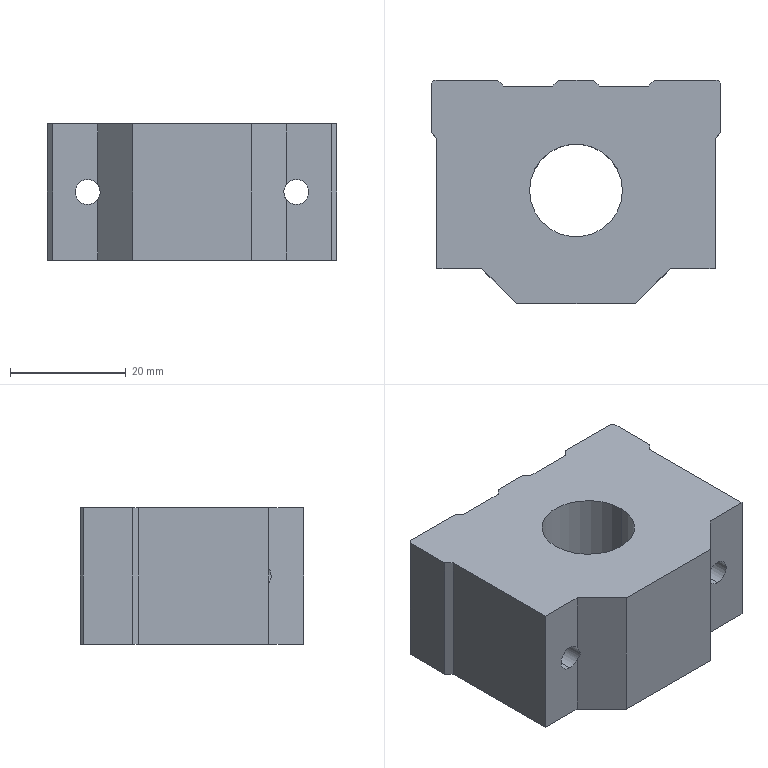Part | SolidWorks | features Extrusion 1, ICE 1 | 1 solid | 30 faces | box 50 x 38.5 x 23.5 mm | volume 34722 mm3 | plane 24 | cylinder 6 | commonest cylinder face diameters 4.3 x4 16 x2
STEP:
#1=CARTESIAN_POINT('',(18.,-13.5,9.6));
#2=VERTEX_POINT('',#1);
#3=CARTESIAN_POINT('',(16.25,-13.5,10.501));
#4=VERTEX_POINT('',#3);
#5=CARTESIAN_POINT('',(18.,-13.5,11.75));
#6=DIRECTION('',(0.,1.,0.));
#7=DIRECTION('',(0.,0.,1.));
#8=AXIS2_PLACEMENT_3D('',#5,#6,#7);
#9=CIRCLE('',#8,2.15);
#10=EDGE_CURVE('',#2,#4,#9,.T.);
#11=ORIENTED_EDGE('',*,*,#10,.F.);
#12=CARTESIAN_POINT('',(18.,19.,9.6));
#13=VERTEX_POINT('',#12);
#14=CARTESIAN_POINT('',(18.,-19.5,9.6));
#15=DIRECTION('',(0.,1.,0.));
#16=VECTOR('',#15,1000.);
#17=LINE('',#14,#16);
#18=EDGE_CURVE('',#2,#13,#17,.T.);
#19=ORIENTED_EDGE('',*,*,#18,.T.);
#20=CARTESIAN_POINT('',(18.,19.,13.9));
#21=VERTEX_POINT('',#20);
#22=CARTESIAN_POINT('',(18.,19.,11.75));
#23=DIRECTION('',(0.,1.,0.));
#24=DIRECTION('',(0.,0.,1.));
#25=AXIS2_PLACEMENT_3D('',#22,#23,#24);
#26=CIRCLE('',#25,2.15);
#27=EDGE_CURVE('',#13,#21,#26,.T.);
#28=ORIENTED_EDGE('',*,*,#27,.T.);
#29=CARTESIAN_POINT('',(18.,-13.5,13.9));
#30=VERTEX_POINT('',#29);
#31=CARTESIAN_POINT('',(18.,-19.5,13.9));
#32=DIRECTION('',(0.,1.,0.));
#33=VECTOR('',#32,1000.);
#34=LINE('',#31,#33);
#35=EDGE_CURVE('',#30,#21,#34,.T.);
#36=ORIENTED_EDGE('',*,*,#35,.F.);
#37=CARTESIAN_POINT('',(16.25,-13.5,12.999));
#38=VERTEX_POINT('',#37);
#39=CARTESIAN_POINT('',(18.,-13.5,11.75));
#40=DIRECTION('',(0.,1.,0.));
#41=DIRECTION('',(0.,0.,1.));
#42=AXIS2_PLACEMENT_3D('',#39,#40,#41);
#43=CIRCLE('',#42,2.15);
#44=EDGE_CURVE('',#38,#30,#43,.T.);
#45=ORIENTED_EDGE('',*,*,#44,.F.);
#46=CARTESIAN_POINT('',(16.25,-13.5,10.501));
#47=CARTESIAN_POINT('',(15.698,-14.052,11.275));
#48=CARTESIAN_POINT('',(15.698,-14.052,12.225));
#49=CARTESIAN_POINT('',(16.25,-13.5,12.999));
#50=(BOUNDED_CURVE()B_SPLINE_CURVE(3,(#46,#47,#48,#49),.UNSPECIFIED.,.F.,.F.)B_SPLINE_CURVE_WITH_KNOTS((4,4),(2.522,3.761),.UNSPECIFIED.)CURVE()GEOMETRIC_REPRESENTATION_ITEM()RATIONAL_B_SPLINE_CURVE((1.,0.876,0.876,1.))REPRESENTATION_ITEM(''));
#51=EDGE_CURVE('',#4,#38,#50,.T.);
#52=ORIENTED_EDGE('',*,*,#51,.F.);
#53=EDGE_LOOP('',(#11,#19,#28,#36,#45,#52));
#54=FACE_OUTER_BOUND('',#53,.T.);
#55=CARTESIAN_POINT('',(18.,-19.5,11.75));
#56=DIRECTION('',(0.,1.,0.));
#57=DIRECTION('',(0.,0.,1.));
#58=AXIS2_PLACEMENT_3D('',#55,#56,#57);
#59=CYLINDRICAL_SURFACE('',#58,2.15);
#60=ADVANCED_FACE('',(#54),#59,.F.);
#61=CARTESIAN_POINT('',(-18.,-13.5,9.6));
#62=VERTEX_POINT('',#61);
#63=CARTESIAN_POINT('',(-18.,-13.5,13.9));
#64=VERTEX_POINT('',#63);
#65=CARTESIAN_POINT('',(-18.,-13.5,11.75));
#66=DIRECTION('',(0.,1.,0.));
#67=DIRECTION('',(0.,0.,1.));
#68=AXIS2_PLACEMENT_3D('',#65,#66,#67);
#69=CIRCLE('',#68,2.15);
#70=EDGE_CURVE('',#62,#64,#69,.T.);
#71=ORIENTED_EDGE('',*,*,#70,.F.);
#72=CARTESIAN_POINT('',(-18.,19.,9.6));
#73=VERTEX_POINT('',#72);
#74=CARTESIAN_POINT('',(-18.,-19.5,9.6));
#75=DIRECTION('',(0.,1.,0.));
#76=VECTOR('',#75,1000.);
#77=LINE('',#74,#76);
#78=EDGE_CURVE('',#62,#73,#77,.T.);
#79=ORIENTED_EDGE('',*,*,#78,.T.);
#80=CARTESIAN_POINT('',(-18.,19.,13.9));
#81=VERTEX_POINT('',#80);
#82=CARTESIAN_POINT('',(-18.,19.,11.75));
#83=DIRECTION('',(0.,1.,0.));
#84=DIRECTION('',(0.,0.,1.));
#85=AXIS2_PLACEMENT_3D('',#82,#83,#84);
#86=CIRCLE('',#85,2.15);
#87=EDGE_CURVE('',#73,#81,#86,.T.);
#88=ORIENTED_EDGE('',*,*,#87,.T.);
#89=CARTESIAN_POINT('',(-18.,-19.5,13.9));
#90=DIRECTION('',(0.,1.,0.));
#91=VECTOR('',#90,1000.);
#92=LINE('',#89,#91);
#93=EDGE_CURVE('',#64,#81,#92,.T.);
#94=ORIENTED_EDGE('',*,*,#93,.F.);
#95=EDGE_LOOP('',(#71,#79,#88,#94));
#96=FACE_OUTER_BOUND('',#95,.T.);
#97=CARTESIAN_POINT('',(-18.,-19.5,11.75));
#98=DIRECTION('',(0.,1.,0.));
#99=DIRECTION('',(0.,0.,1.));
#100=AXIS2_PLACEMENT_3D('',#97,#98,#99);
#101=CYLINDRICAL_SURFACE('',#100,2.15);
#102=ADVANCED_FACE('',(#96),#101,.F.);
#103=CARTESIAN_POINT('',(-8.,0.,23.5));
#104=VERTEX_POINT('',#103);
#105=CARTESIAN_POINT('',(8.,0.,23.5));
#106=VERTEX_POINT('',#105);
#107=CARTESIAN_POINT('',(0.,0.,23.5));
#108=DIRECTION('',(0.,0.,1.));
#109=DIRECTION('',(1.,0.,0.));
#110=AXIS2_PLACEMENT_3D('',#107,#108,#109);
#111=CIRCLE('',#110,8.);
#112=EDGE_CURVE('',#104,#106,#111,.T.);
#113=ORIENTED_EDGE('',*,*,#112,.T.);
#114=CARTESIAN_POINT('',(8.,0.,0.));
#115=VERTEX_POINT('',#114);
#116=CARTESIAN_POINT('',(8.,0.,23.5));
#117=DIRECTION('',(0.,0.,-1.));
#118=VECTOR('',#117,1000.);
#119=LINE('',#116,#118);
#120=EDGE_CURVE('',#106,#115,#119,.T.);
#121=ORIENTED_EDGE('',*,*,#120,.T.);
#122=CARTESIAN_POINT('',(-8.,0.,0.));
#123=VERTEX_POINT('',#122);
#124=CARTESIAN_POINT('',(0.,0.,0.));
#125=DIRECTION('',(0.,0.,1.));
#126=DIRECTION('',(1.,0.,0.));
#127=AXIS2_PLACEMENT_3D('',#124,#125,#126);
#128=CIRCLE('',#127,8.);
#129=EDGE_CURVE('',#123,#115,#128,.T.);
#130=ORIENTED_EDGE('',*,*,#129,.F.);
#131=CARTESIAN_POINT('',(-8.,0.,23.5));
#132=DIRECTION('',(0.,0.,-1.));
#133=VECTOR('',#132,1000.);
#134=LINE('',#131,#133);
#135=EDGE_CURVE('',#104,#123,#134,.T.);
#136=ORIENTED_EDGE('',*,*,#135,.F.);
#137=EDGE_LOOP('',(#113,#121,#130,#136));
#138=FACE_OUTER_BOUND('',#137,.T.);
#139=CARTESIAN_POINT('',(0.,0.,23.5));
#140=DIRECTION('',(0.,0.,-1.));
#141=DIRECTION('',(-1.,0.,0.));
#142=AXIS2_PLACEMENT_3D('',#139,#140,#141);
#143=CYLINDRICAL_SURFACE('',#142,8.);
#144=ADVANCED_FACE('',(#138),#143,.F.);
#145=CARTESIAN_POINT('',(-16.25,-13.5,23.5));
#146=VERTEX_POINT('',#145);
#147=CARTESIAN_POINT('',(-10.25,-19.5,23.5));
#148=VERTEX_POINT('',#147);
#149=CARTESIAN_POINT('',(-16.25,-13.5,23.5));
#150=DIRECTION('',(0.7071,-0.7071,0.));
#151=VECTOR('',#150,1000.);
#152=LINE('',#149,#151);
#153=EDGE_CURVE('',#146,#148,#152,.T.);
#154=ORIENTED_EDGE('',*,*,#153,.T.);
#155=CARTESIAN_POINT('',(10.25,-19.5,23.5));
#156=VERTEX_POINT('',#155);
#157=CARTESIAN_POINT('',(-10.25,-19.5,23.5));
#158=DIRECTION('',(1.,0.,0.));
#159=VECTOR('',#158,1000.);
#160=LINE('',#157,#159);
#161=EDGE_CURVE('',#148,#156,#160,.T.);
#162=ORIENTED_EDGE('',*,*,#161,.T.);
#163=CARTESIAN_POINT('',(16.25,-13.5,23.5));
#164=VERTEX_POINT('',#163);
#165=CARTESIAN_POINT('',(16.25,-13.5,23.5));
#166=DIRECTION('',(0.7071,0.7071,0.));
#167=VECTOR('',#166,1000.);
#168=LINE('',#165,#167);
#169=EDGE_CURVE('',#156,#164,#168,.T.);
#170=ORIENTED_EDGE('',*,*,#169,.T.);
#171=CARTESIAN_POINT('',(24.,-13.5,23.5));
#172=VERTEX_POINT('',#171);
#173=CARTESIAN_POINT('',(16.25,-13.5,23.5));
#174=DIRECTION('',(1.,0.,0.));
#175=VECTOR('',#174,1000.);
#176=LINE('',#173,#175);
#177=EDGE_CURVE('',#164,#172,#176,.T.);
#178=ORIENTED_EDGE('',*,*,#177,.T.);
#179=CARTESIAN_POINT('',(24.,9.,23.5));
#180=VERTEX_POINT('',#179);
#181=CARTESIAN_POINT('',(24.,-13.5,23.5));
#182=DIRECTION('',(0.,1.,0.));
#183=VECTOR('',#182,1000.);
#184=LINE('',#181,#183);
#185=EDGE_CURVE('',#172,#180,#184,.T.);
#186=ORIENTED_EDGE('',*,*,#185,.T.);
#187=CARTESIAN_POINT('',(25.,10.,23.5));
#188=VERTEX_POINT('',#187);
#189=CARTESIAN_POINT('',(24.,9.,23.5));
#190=DIRECTION('',(0.7071,0.7071,0.));
#191=VECTOR('',#190,1000.);
#192=LINE('',#189,#191);
#193=EDGE_CURVE('',#180,#188,#192,.T.);
#194=ORIENTED_EDGE('',*,*,#193,.T.);
#195=CARTESIAN_POINT('',(25.,18.5,23.5));
#196=VERTEX_POINT('',#195);
#197=CARTESIAN_POINT('',(25.,10.,23.5));
#198=DIRECTION('',(0.,1.,0.));
#199=VECTOR('',#198,1000.);
#200=LINE('',#197,#199);
#201=EDGE_CURVE('',#188,#196,#200,.T.);
#202=ORIENTED_EDGE('',*,*,#201,.T.);
#203=CARTESIAN_POINT('',(24.5,19.,23.5));
#204=VERTEX_POINT('',#203);
#205=CARTESIAN_POINT('',(25.,18.5,23.5));
#206=DIRECTION('',(-0.7071,0.7071,0.));
#207=VECTOR('',#206,1000.);
#208=LINE('',#205,#207);
#209=EDGE_CURVE('',#196,#204,#208,.T.);
#210=ORIENTED_EDGE('',*,*,#209,.T.);
#211=CARTESIAN_POINT('',(13.5,19.,23.5));
#212=VERTEX_POINT('',#211);
#213=CARTESIAN_POINT('',(24.5,19.,23.5));
#214=DIRECTION('',(-1.,0.,0.));
#215=VECTOR('',#214,1000.);
#216=LINE('',#213,#215);
#217=EDGE_CURVE('',#204,#212,#216,.T.);
#218=ORIENTED_EDGE('',*,*,#217,.T.);
#219=CARTESIAN_POINT('',(12.5,18.,23.5));
#220=VERTEX_POINT('',#219);
#221=CARTESIAN_POINT('',(13.5,19.,23.5));
#222=DIRECTION('',(-0.7071,-0.7071,0.));
#223=VECTOR('',#222,1000.);
#224=LINE('',#221,#223);
#225=EDGE_CURVE('',#212,#220,#224,.T.);
#226=ORIENTED_EDGE('',*,*,#225,.T.);
#227=CARTESIAN_POINT('',(4.,18.,23.5));
#228=VERTEX_POINT('',#227);
#229=CARTESIAN_POINT('',(12.5,18.,23.5));
#230=DIRECTION('',(-1.,0.,0.));
#231=VECTOR('',#230,1000.);
#232=LINE('',#229,#231);
#233=EDGE_CURVE('',#220,#228,#232,.T.);
#234=ORIENTED_EDGE('',*,*,#233,.T.);
#235=CARTESIAN_POINT('',(3.,19.,23.5));
#236=VERTEX_POINT('',#235);
#237=CARTESIAN_POINT('',(4.,18.,23.5));
#238=DIRECTION('',(-0.7071,0.7071,0.));
#239=VECTOR('',#238,1000.);
#240=LINE('',#237,#239);
#241=EDGE_CURVE('',#228,#236,#240,.T.);
#242=ORIENTED_EDGE('',*,*,#241,.T.);
#243=CARTESIAN_POINT('',(-3.,19.,23.5));
#244=VERTEX_POINT('',#243);
#245=CARTESIAN_POINT('',(3.,19.,23.5));
#246=DIRECTION('',(-1.,0.,0.));
#247=VECTOR('',#246,1000.);
#248=LINE('',#245,#247);
#249=EDGE_CURVE('',#236,#244,#248,.T.);
#250=ORIENTED_EDGE('',*,*,#249,.T.);
#251=CARTESIAN_POINT('',(-4.,18.,23.5));
#252=VERTEX_POINT('',#251);
#253=CARTESIAN_POINT('',(-3.,19.,23.5));
#254=DIRECTION('',(-0.7071,-0.7071,0.));
#255=VECTOR('',#254,1000.);
#256=LINE('',#253,#255);
#257=EDGE_CURVE('',#244,#252,#256,.T.);
#258=ORIENTED_EDGE('',*,*,#257,.T.);
#259=CARTESIAN_POINT('',(-12.5,18.,23.5));
#260=VERTEX_POINT('',#259);
#261=CARTESIAN_POINT('',(-4.,18.,23.5));
#262=DIRECTION('',(-1.,0.,0.));
#263=VECTOR('',#262,1000.);
#264=LINE('',#261,#263);
#265=EDGE_CURVE('',#252,#260,#264,.T.);
#266=ORIENTED_EDGE('',*,*,#265,.T.);
#267=CARTESIAN_POINT('',(-13.5,19.,23.5));
#268=VERTEX_POINT('',#267);
#269=CARTESIAN_POINT('',(-12.5,18.,23.5));
#270=DIRECTION('',(-0.7071,0.7071,0.));
#271=VECTOR('',#270,1000.);
#272=LINE('',#269,#271);
#273=EDGE_CURVE('',#260,#268,#272,.T.);
#274=ORIENTED_EDGE('',*,*,#273,.T.);
#275=CARTESIAN_POINT('',(-24.5,19.,23.5));
#276=VERTEX_POINT('',#275);
#277=CARTESIAN_POINT('',(-13.5,19.,23.5));
#278=DIRECTION('',(-1.,0.,0.));
#279=VECTOR('',#278,1000.);
#280=LINE('',#277,#279);
#281=EDGE_CURVE('',#268,#276,#280,.T.);
#282=ORIENTED_EDGE('',*,*,#281,.T.);
#283=CARTESIAN_POINT('',(-25.,18.5,23.5));
#284=VERTEX_POINT('',#283);
#285=CARTESIAN_POINT('',(-24.5,19.,23.5));
#286=DIRECTION('',(-0.7071,-0.7071,0.));
#287=VECTOR('',#286,1000.);
#288=LINE('',#285,#287);
#289=EDGE_CURVE('',#276,#284,#288,.T.);
#290=ORIENTED_EDGE('',*,*,#289,.T.);
#291=CARTESIAN_POINT('',(-25.,10.,23.5));
#292=VERTEX_POINT('',#291);
#293=CARTESIAN_POINT('',(-25.,18.5,23.5));
#294=DIRECTION('',(0.,-1.,0.));
#295=VECTOR('',#294,1000.);
#296=LINE('',#293,#295);
#297=EDGE_CURVE('',#284,#292,#296,.T.);
#298=ORIENTED_EDGE('',*,*,#297,.T.);
#299=CARTESIAN_POINT('',(-24.,9.,23.5));
#300=VERTEX_POINT('',#299);
#301=CARTESIAN_POINT('',(-25.,10.,23.5));
#302=DIRECTION('',(0.7071,-0.7071,0.));
#303=VECTOR('',#302,1000.);
#304=LINE('',#301,#303);
#305=EDGE_CURVE('',#292,#300,#304,.T.);
#306=ORIENTED_EDGE('',*,*,#305,.T.);
#307=CARTESIAN_POINT('',(-24.,-13.5,23.5));
#308=VERTEX_POINT('',#307);
#309=CARTESIAN_POINT('',(-24.,9.,23.5));
#310=DIRECTION('',(0.,-1.,0.));
#311=VECTOR('',#310,1000.);
#312=LINE('',#309,#311);
#313=EDGE_CURVE('',#300,#308,#312,.T.);
#314=ORIENTED_EDGE('',*,*,#313,.T.);
#315=CARTESIAN_POINT('',(-24.,-13.5,23.5));
#316=DIRECTION('',(1.,0.,0.));
#317=VECTOR('',#316,1000.);
#318=LINE('',#315,#317);
#319=EDGE_CURVE('',#308,#146,#318,.T.);
#320=ORIENTED_EDGE('',*,*,#319,.T.);
#321=EDGE_LOOP('',(#154,#162,#170,#178,#186,#194,#202,#210,#218,#226,#234,#242,#250,#258,#266,#274,#282,#290,#298,#306,#314,#320));
#322=FACE_OUTER_BOUND('',#321,.T.);
#323=ORIENTED_EDGE('',*,*,#112,.F.);
#324=CARTESIAN_POINT('',(0.,0.,23.5));
#325=DIRECTION('',(0.,0.,1.));
#326=DIRECTION('',(1.,0.,0.));
#327=AXIS2_PLACEMENT_3D('',#324,#325,#326);
#328=CIRCLE('',#327,8.);
#329=EDGE_CURVE('',#106,#104,#328,.T.);
#330=ORIENTED_EDGE('',*,*,#329,.F.);
#331=EDGE_LOOP('',(#323,#330));
#332=FACE_BOUND('',#331,.T.);
#333=CARTESIAN_POINT('',(0.,0.,23.5));
#334=DIRECTION('',(0.,0.,-1.));
#335=DIRECTION('',(-1.,0.,0.));
#336=AXIS2_PLACEMENT_3D('',#333,#334,#335);
#337=PLANE('',#336);
#338=ADVANCED_FACE('',(#322,#332),#337,.F.);
#339=CARTESIAN_POINT('',(-16.25,-13.5,0.));
#340=VERTEX_POINT('',#339);
#341=CARTESIAN_POINT('',(-10.25,-19.5,0.));
#342=VERTEX_POINT('',#341);
#343=CARTESIAN_POINT('',(-16.25,-13.5,0.));
#344=DIRECTION('',(0.7071,-0.7071,0.));
#345=VECTOR('',#344,1000.);
#346=LINE('',#343,#345);
#347=EDGE_CURVE('',#340,#342,#346,.T.);
#348=ORIENTED_EDGE('',*,*,#347,.F.);
#349=CARTESIAN_POINT('',(-24.,-13.5,0.));
#350=VERTEX_POINT('',#349);
#351=CARTESIAN_POINT('',(-24.,-13.5,0.));
#352=DIRECTION('',(1.,0.,0.));
#353=VECTOR('',#352,1000.);
#354=LINE('',#351,#353);
#355=EDGE_CURVE('',#350,#340,#354,.T.);
#356=ORIENTED_EDGE('',*,*,#355,.F.);
#357=CARTESIAN_POINT('',(-24.,9.,0.));
#358=VERTEX_POINT('',#357);
#359=CARTESIAN_POINT('',(-24.,9.,0.));
#360=DIRECTION('',(0.,-1.,0.));
#361=VECTOR('',#360,1000.);
#362=LINE('',#359,#361);
#363=EDGE_CURVE('',#358,#350,#362,.T.);
#364=ORIENTED_EDGE('',*,*,#363,.F.);
#365=CARTESIAN_POINT('',(-25.,10.,0.));
#366=VERTEX_POINT('',#365);
#367=CARTESIAN_POINT('',(-25.,10.,0.));
#368=DIRECTION('',(0.7071,-0.7071,0.));
#369=VECTOR('',#368,1000.);
#370=LINE('',#367,#369);
#371=EDGE_CURVE('',#366,#358,#370,.T.);
#372=ORIENTED_EDGE('',*,*,#371,.F.);
#373=CARTESIAN_POINT('',(-25.,18.5,0.));
#374=VERTEX_POINT('',#373);
#375=CARTESIAN_POINT('',(-25.,18.5,0.));
#376=DIRECTION('',(0.,-1.,0.));
#377=VECTOR('',#376,1000.);
#378=LINE('',#375,#377);
#379=EDGE_CURVE('',#374,#366,#378,.T.);
#380=ORIENTED_EDGE('',*,*,#379,.F.);
#381=CARTESIAN_POINT('',(-24.5,19.,0.));
#382=VERTEX_POINT('',#381);
#383=CARTESIAN_POINT('',(-24.5,19.,0.));
#384=DIRECTION('',(-0.7071,-0.7071,0.));
#385=VECTOR('',#384,1000.);
#386=LINE('',#383,#385);
#387=EDGE_CURVE('',#382,#374,#386,.T.);
#388=ORIENTED_EDGE('',*,*,#387,.F.);
#389=CARTESIAN_POINT('',(-13.5,19.,0.));
#390=VERTEX_POINT('',#389);
#391=CARTESIAN_POINT('',(-13.5,19.,0.));
#392=DIRECTION('',(-1.,0.,0.));
#393=VECTOR('',#392,1000.);
#394=LINE('',#391,#393);
#395=EDGE_CURVE('',#390,#382,#394,.T.);
#396=ORIENTED_EDGE('',*,*,#395,.F.);
#397=CARTESIAN_POINT('',(-12.5,18.,0.));
#398=VERTEX_POINT('',#397);
#399=CARTESIAN_POINT('',(-12.5,18.,0.));
#400=DIRECTION('',(-0.7071,0.7071,0.));
#401=VECTOR('',#400,1000.);
#402=LINE('',#399,#401);
#403=EDGE_CURVE('',#398,#390,#402,.T.);
#404=ORIENTED_EDGE('',*,*,#403,.F.);
#405=CARTESIAN_POINT('',(-4.,18.,0.));
#406=VERTEX_POINT('',#405);
#407=CARTESIAN_POINT('',(-4.,18.,0.));
#408=DIRECTION('',(-1.,0.,0.));
#409=VECTOR('',#408,1000.);
#410=LINE('',#407,#409);
#411=EDGE_CURVE('',#406,#398,#410,.T.);
#412=ORIENTED_EDGE('',*,*,#411,.F.);
#413=CARTESIAN_POINT('',(-3.,19.,0.));
#414=VERTEX_POINT('',#413);
#415=CARTESIAN_POINT('',(-3.,19.,0.));
#416=DIRECTION('',(-0.7071,-0.7071,0.));
#417=VECTOR('',#416,1000.);
#418=LINE('',#415,#417);
#419=EDGE_CURVE('',#414,#406,#418,.T.);
#420=ORIENTED_EDGE('',*,*,#419,.F.);
#421=CARTESIAN_POINT('',(3.,19.,0.));
#422=VERTEX_POINT('',#421);
#423=CARTESIAN_POINT('',(3.,19.,0.));
#424=DIRECTION('',(-1.,0.,0.));
#425=VECTOR('',#424,1000.);
#426=LINE('',#423,#425);
#427=EDGE_CURVE('',#422,#414,#426,.T.);
#428=ORIENTED_EDGE('',*,*,#427,.F.);
#429=CARTESIAN_POINT('',(4.,18.,0.));
#430=VERTEX_POINT('',#429);
#431=CARTESIAN_POINT('',(4.,18.,0.));
#432=DIRECTION('',(-0.7071,0.7071,0.));
#433=VECTOR('',#432,1000.);
#434=LINE('',#431,#433);
#435=EDGE_CURVE('',#430,#422,#434,.T.);
#436=ORIENTED_EDGE('',*,*,#435,.F.);
#437=CARTESIAN_POINT('',(12.5,18.,0.));
#438=VERTEX_POINT('',#437);
#439=CARTESIAN_POINT('',(12.5,18.,0.));
#440=DIRECTION('',(-1.,0.,0.));
#441=VECTOR('',#440,1000.);
#442=LINE('',#439,#441);
#443=EDGE_CURVE('',#438,#430,#442,.T.);
#444=ORIENTED_EDGE('',*,*,#443,.F.);
#445=CARTESIAN_POINT('',(13.5,19.,0.));
#446=VERTEX_POINT('',#445);
#447=CARTESIAN_POINT('',(13.5,19.,0.));
#448=DIRECTION('',(-0.7071,-0.7071,0.));
#449=VECTOR('',#448,1000.);
#450=LINE('',#447,#449);
#451=EDGE_CURVE('',#446,#438,#450,.T.);
#452=ORIENTED_EDGE('',*,*,#451,.F.);
#453=CARTESIAN_POINT('',(24.5,19.,0.));
#454=VERTEX_POINT('',#453);
#455=CARTESIAN_POINT('',(24.5,19.,0.));
#456=DIRECTION('',(-1.,0.,0.));
#457=VECTOR('',#456,1000.);
#458=LINE('',#455,#457);
#459=EDGE_CURVE('',#454,#446,#458,.T.);
#460=ORIENTED_EDGE('',*,*,#459,.F.);
#461=CARTESIAN_POINT('',(25.,18.5,0.));
#462=VERTEX_POINT('',#461);
#463=CARTESIAN_POINT('',(25.,18.5,0.));
#464=DIRECTION('',(-0.7071,0.7071,0.));
#465=VECTOR('',#464,1000.);
#466=LINE('',#463,#465);
#467=EDGE_CURVE('',#462,#454,#466,.T.);
#468=ORIENTED_EDGE('',*,*,#467,.F.);
#469=CARTESIAN_POINT('',(25.,10.,0.));
#470=VERTEX_POINT('',#469);
#471=CARTESIAN_POINT('',(25.,10.,0.));
#472=DIRECTION('',(0.,1.,0.));
#473=VECTOR('',#472,1000.);
#474=LINE('',#471,#473);
#475=EDGE_CURVE('',#470,#462,#474,.T.);
#476=ORIENTED_EDGE('',*,*,#475,.F.);
#477=CARTESIAN_POINT('',(24.,9.,0.));
#478=VERTEX_POINT('',#477);
#479=CARTESIAN_POINT('',(24.,9.,0.));
#480=DIRECTION('',(0.7071,0.7071,0.));
#481=VECTOR('',#480,1000.);
#482=LINE('',#479,#481);
#483=EDGE_CURVE('',#478,#470,#482,.T.);
#484=ORIENTED_EDGE('',*,*,#483,.F.);
#485=CARTESIAN_POINT('',(24.,-13.5,0.));
#486=VERTEX_POINT('',#485);
#487=CARTESIAN_POINT('',(24.,-13.5,0.));
#488=DIRECTION('',(0.,1.,0.));
#489=VECTOR('',#488,1000.);
#490=LINE('',#487,#489);
#491=EDGE_CURVE('',#486,#478,#490,.T.);
#492=ORIENTED_EDGE('',*,*,#491,.F.);
#493=CARTESIAN_POINT('',(16.25,-13.5,0.));
#494=VERTEX_POINT('',#493);
#495=CARTESIAN_POINT('',(16.25,-13.5,0.));
#496=DIRECTION('',(1.,0.,0.));
#497=VECTOR('',#496,1000.);
#498=LINE('',#495,#497);
#499=EDGE_CURVE('',#494,#486,#498,.T.);
#500=ORIENTED_EDGE('',*,*,#499,.F.);
#501=CARTESIAN_POINT('',(10.25,-19.5,0.));
#502=VERTEX_POINT('',#501);
#503=CARTESIAN_POINT('',(16.25,-13.5,0.));
#504=DIRECTION('',(0.7071,0.7071,0.));
#505=VECTOR('',#504,1000.);
#506=LINE('',#503,#505);
#507=EDGE_CURVE('',#502,#494,#506,.T.);
#508=ORIENTED_EDGE('',*,*,#507,.F.);
#509=CARTESIAN_POINT('',(-10.25,-19.5,0.));
#510=DIRECTION('',(1.,0.,0.));
#511=VECTOR('',#510,1000.);
#512=LINE('',#509,#511);
#513=EDGE_CURVE('',#342,#502,#512,.T.);
#514=ORIENTED_EDGE('',*,*,#513,.F.);
#515=EDGE_LOOP('',(#348,#356,#364,#372,#380,#388,#396,#404,#412,#420,#428,#436,#444,#452,#460,#468,#476,#484,#492,#500,#508,#514));
#516=FACE_OUTER_BOUND('',#515,.T.);
#517=ORIENTED_EDGE('',*,*,#129,.T.);
#518=CARTESIAN_POINT('',(0.,0.,0.));
#519=DIRECTION('',(0.,0.,1.));
#520=DIRECTION('',(1.,0.,0.));
#521=AXIS2_PLACEMENT_3D('',#518,#519,#520);
#522=CIRCLE('',#521,8.);
#523=EDGE_CURVE('',#115,#123,#522,.T.);
#524=ORIENTED_EDGE('',*,*,#523,.T.);
#525=EDGE_LOOP('',(#517,#524));
#526=FACE_BOUND('',#525,.T.);
#527=CARTESIAN_POINT('',(0.,0.,0.));
#528=DIRECTION('',(0.,0.,-1.));
#529=DIRECTION('',(-1.,0.,0.));
#530=AXIS2_PLACEMENT_3D('',#527,#528,#529);
#531=PLANE('',#530);
#532=ADVANCED_FACE('',(#516,#526),#531,.T.);
#533=CARTESIAN_POINT('',(-16.25,-13.5,12.999));
#534=VERTEX_POINT('',#533);
#535=CARTESIAN_POINT('',(-16.25,-13.5,23.5));
#536=DIRECTION('',(0.,0.,-1.));
#537=VECTOR('',#536,1000.);
#538=LINE('',#535,#537);
#539=EDGE_CURVE('',#146,#534,#538,.T.);
#540=ORIENTED_EDGE('',*,*,#539,.T.);
#541=CARTESIAN_POINT('',(-16.25,-13.5,10.501));
#542=VERTEX_POINT('',#541);
#543=CARTESIAN_POINT('',(-16.25,-13.5,12.999));
#544=CARTESIAN_POINT('',(-15.698,-14.052,12.225));
#545=CARTESIAN_POINT('',(-15.698,-14.052,11.275));
#546=CARTESIAN_POINT('',(-16.25,-13.5,10.501));
#547=(BOUNDED_CURVE()B_SPLINE_CURVE(3,(#543,#544,#545,#546),.UNSPECIFIED.,.F.,.F.)B_SPLINE_CURVE_WITH_KNOTS((4,4),(2.522,3.761),.UNSPECIFIED.)CURVE()GEOMETRIC_REPRESENTATION_ITEM()RATIONAL_B_SPLINE_CURVE((1.,0.876,0.876,1.))REPRESENTATION_ITEM(''));
#548=EDGE_CURVE('',#534,#542,#547,.T.);
#549=ORIENTED_EDGE('',*,*,#548,.T.);
#550=CARTESIAN_POINT('',(-16.25,-13.5,23.5));
#551=DIRECTION('',(0.,0.,-1.));
#552=VECTOR('',#551,1000.);
#553=LINE('',#550,#552);
#554=EDGE_CURVE('',#542,#340,#553,.T.);
#555=ORIENTED_EDGE('',*,*,#554,.T.);
#556=ORIENTED_EDGE('',*,*,#347,.T.);
#557=CARTESIAN_POINT('',(-10.25,-19.5,23.5));
#558=DIRECTION('',(0.,0.,-1.));
#559=VECTOR('',#558,1000.);
#560=LINE('',#557,#559);
#561=EDGE_CURVE('',#148,#342,#560,.T.);
#562=ORIENTED_EDGE('',*,*,#561,.F.);
#563=ORIENTED_EDGE('',*,*,#153,.F.);
#564=EDGE_LOOP('',(#540,#549,#555,#556,#562,#563));
#565=FACE_OUTER_BOUND('',#564,.T.);
#566=CARTESIAN_POINT('',(-16.25,-13.5,23.5));
#567=DIRECTION('',(0.7071,0.7071,0.));
#568=DIRECTION('',(-0.7071,0.7071,0.));
#569=AXIS2_PLACEMENT_3D('',#566,#567,#568);
#570=PLANE('',#569);
#571=ADVANCED_FACE('',(#565),#570,.F.);
#572=ORIENTED_EDGE('',*,*,#513,.T.);
#573=CARTESIAN_POINT('',(10.25,-19.5,23.5));
#574=DIRECTION('',(0.,0.,-1.));
#575=VECTOR('',#574,1000.);
#576=LINE('',#573,#575);
#577=EDGE_CURVE('',#156,#502,#576,.T.);
#578=ORIENTED_EDGE('',*,*,#577,.F.);
#579=ORIENTED_EDGE('',*,*,#161,.F.);
#580=ORIENTED_EDGE('',*,*,#561,.T.);
#581=EDGE_LOOP('',(#572,#578,#579,#580));
#582=FACE_OUTER_BOUND('',#581,.T.);
#583=CARTESIAN_POINT('',(-10.25,-19.5,23.5));
#584=DIRECTION('',(0.,1.,0.));
#585=DIRECTION('',(-1.,0.,0.));
#586=AXIS2_PLACEMENT_3D('',#583,#584,#585);
#587=PLANE('',#586);
#588=ADVANCED_FACE('',(#582),#587,.F.);
#589=CARTESIAN_POINT('',(16.25,-13.5,23.5));
#590=DIRECTION('',(0.,0.,-1.));
#591=VECTOR('',#590,1000.);
#592=LINE('',#589,#591);
#593=EDGE_CURVE('',#4,#494,#592,.T.);
#594=ORIENTED_EDGE('',*,*,#593,.F.);
#595=ORIENTED_EDGE('',*,*,#51,.T.);
#596=CARTESIAN_POINT('',(16.25,-13.5,23.5));
#597=DIRECTION('',(0.,0.,-1.));
#598=VECTOR('',#597,1000.);
#599=LINE('',#596,#598);
#600=EDGE_CURVE('',#164,#38,#599,.T.);
#601=ORIENTED_EDGE('',*,*,#600,.F.);
#602=ORIENTED_EDGE('',*,*,#169,.F.);
#603=ORIENTED_EDGE('',*,*,#577,.T.);
#604=ORIENTED_EDGE('',*,*,#507,.T.);
#605=EDGE_LOOP('',(#594,#595,#601,#602,#603,#604));
#606=FACE_OUTER_BOUND('',#605,.T.);
#607=CARTESIAN_POINT('',(16.25,-13.5,23.5));
#608=DIRECTION('',(-0.7071,0.7071,0.));
#609=DIRECTION('',(-0.7071,-0.7071,0.));
#610=AXIS2_PLACEMENT_3D('',#607,#608,#609);
#611=PLANE('',#610);
#612=ADVANCED_FACE('',(#606),#611,.F.);
#613=ORIENTED_EDGE('',*,*,#600,.T.);
#614=ORIENTED_EDGE('',*,*,#44,.T.);
#615=CARTESIAN_POINT('',(18.,-13.5,11.75));
#616=DIRECTION('',(0.,1.,0.));
#617=DIRECTION('',(0.,0.,1.));
#618=AXIS2_PLACEMENT_3D('',#615,#616,#617);
#619=CIRCLE('',#618,2.15);
#620=EDGE_CURVE('',#30,#2,#619,.T.);
#621=ORIENTED_EDGE('',*,*,#620,.T.);
#622=ORIENTED_EDGE('',*,*,#10,.T.);
#623=ORIENTED_EDGE('',*,*,#593,.T.);
#624=ORIENTED_EDGE('',*,*,#499,.T.);
#625=CARTESIAN_POINT('',(24.,-13.5,23.5));
#626=DIRECTION('',(0.,0.,-1.));
#627=VECTOR('',#626,1000.);
#628=LINE('',#625,#627);
#629=EDGE_CURVE('',#172,#486,#628,.T.);
#630=ORIENTED_EDGE('',*,*,#629,.F.);
#631=ORIENTED_EDGE('',*,*,#177,.F.);
#632=EDGE_LOOP('',(#613,#614,#621,#622,#623,#624,#630,#631));
#633=FACE_OUTER_BOUND('',#632,.T.);
#634=CARTESIAN_POINT('',(16.25,-13.5,23.5));
#635=DIRECTION('',(0.,1.,0.));
#636=DIRECTION('',(0.,0.,1.));
#637=AXIS2_PLACEMENT_3D('',#634,#635,#636);
#638=PLANE('',#637);
#639=ADVANCED_FACE('',(#633),#638,.F.);
#640=ORIENTED_EDGE('',*,*,#491,.T.);
#641=CARTESIAN_POINT('',(24.,9.,23.5));
#642=DIRECTION('',(0.,0.,-1.));
#643=VECTOR('',#642,1000.);
#644=LINE('',#641,#643);
#645=EDGE_CURVE('',#180,#478,#644,.T.);
#646=ORIENTED_EDGE('',*,*,#645,.F.);
#647=ORIENTED_EDGE('',*,*,#185,.F.);
#648=ORIENTED_EDGE('',*,*,#629,.T.);
#649=EDGE_LOOP('',(#640,#646,#647,#648));
#650=FACE_OUTER_BOUND('',#649,.T.);
#651=CARTESIAN_POINT('',(24.,-13.5,23.5));
#652=DIRECTION('',(-1.,0.,0.));
#653=DIRECTION('',(0.,0.,1.));
#654=AXIS2_PLACEMENT_3D('',#651,#652,#653);
#655=PLANE('',#654);
#656=ADVANCED_FACE('',(#650),#655,.F.);
#657=ORIENTED_EDGE('',*,*,#483,.T.);
#658=CARTESIAN_POINT('',(25.,10.,23.5));
#659=DIRECTION('',(0.,0.,-1.));
#660=VECTOR('',#659,1000.);
#661=LINE('',#658,#660);
#662=EDGE_CURVE('',#188,#470,#661,.T.);
#663=ORIENTED_EDGE('',*,*,#662,.F.);
#664=ORIENTED_EDGE('',*,*,#193,.F.);
#665=ORIENTED_EDGE('',*,*,#645,.T.);
#666=EDGE_LOOP('',(#657,#663,#664,#665));
#667=FACE_OUTER_BOUND('',#666,.T.);
#668=CARTESIAN_POINT('',(24.,9.,23.5));
#669=DIRECTION('',(-0.7071,0.7071,0.));
#670=DIRECTION('',(-0.7071,-0.7071,0.));
#671=AXIS2_PLACEMENT_3D('',#668,#669,#670);
#672=PLANE('',#671);
#673=ADVANCED_FACE('',(#667),#672,.F.);
#674=ORIENTED_EDGE('',*,*,#475,.T.);
#675=CARTESIAN_POINT('',(25.,18.5,23.5));
#676=DIRECTION('',(0.,0.,-1.));
#677=VECTOR('',#676,1000.);
#678=LINE('',#675,#677);
#679=EDGE_CURVE('',#196,#462,#678,.T.);
#680=ORIENTED_EDGE('',*,*,#679,.F.);
#681=ORIENTED_EDGE('',*,*,#201,.F.);
#682=ORIENTED_EDGE('',*,*,#662,.T.);
#683=EDGE_LOOP('',(#674,#680,#681,#682));
#684=FACE_OUTER_BOUND('',#683,.T.);
#685=CARTESIAN_POINT('',(25.,10.,23.5));
#686=DIRECTION('',(-1.,0.,0.));
#687=DIRECTION('',(0.,-1.,0.));
#688=AXIS2_PLACEMENT_3D('',#685,#686,#687);
#689=PLANE('',#688);
#690=ADVANCED_FACE('',(#684),#689,.F.);
#691=ORIENTED_EDGE('',*,*,#467,.T.);
#692=CARTESIAN_POINT('',(24.5,19.,23.5));
#693=DIRECTION('',(0.,0.,-1.));
#694=VECTOR('',#693,1000.);
#695=LINE('',#692,#694);
#696=EDGE_CURVE('',#204,#454,#695,.T.);
#697=ORIENTED_EDGE('',*,*,#696,.F.);
#698=ORIENTED_EDGE('',*,*,#209,.F.);
#699=ORIENTED_EDGE('',*,*,#679,.T.);
#700=EDGE_LOOP('',(#691,#697,#698,#699));
#701=FACE_OUTER_BOUND('',#700,.T.);
#702=CARTESIAN_POINT('',(25.,18.5,23.5));
#703=DIRECTION('',(-0.7071,-0.7071,0.));
#704=DIRECTION('',(0.7071,-0.7071,0.));
#705=AXIS2_PLACEMENT_3D('',#702,#703,#704);
#706=PLANE('',#705);
#707=ADVANCED_FACE('',(#701),#706,.F.);
#708=CARTESIAN_POINT('',(18.,19.,11.75));
#709=DIRECTION('',(0.,1.,0.));
#710=DIRECTION('',(0.,0.,1.));
#711=AXIS2_PLACEMENT_3D('',#708,#709,#710);
#712=CIRCLE('',#711,2.15);
#713=EDGE_CURVE('',#21,#13,#712,.T.);
#714=ORIENTED_EDGE('',*,*,#713,.F.);
#715=ORIENTED_EDGE('',*,*,#27,.F.);
#716=EDGE_LOOP('',(#714,#715));
#717=FACE_BOUND('',#716,.T.);
#718=ORIENTED_EDGE('',*,*,#459,.T.);
#719=CARTESIAN_POINT('',(13.5,19.,23.5));
#720=DIRECTION('',(0.,0.,-1.));
#721=VECTOR('',#720,1000.);
#722=LINE('',#719,#721);
#723=EDGE_CURVE('',#212,#446,#722,.T.);
#724=ORIENTED_EDGE('',*,*,#723,.F.);
#725=ORIENTED_EDGE('',*,*,#217,.F.);
#726=ORIENTED_EDGE('',*,*,#696,.T.);
#727=EDGE_LOOP('',(#718,#724,#725,#726));
#728=FACE_OUTER_BOUND('',#727,.T.);
#729=CARTESIAN_POINT('',(24.5,19.,23.5));
#730=DIRECTION('',(0.,-1.,0.));
#731=DIRECTION('',(0.,0.,-1.));
#732=AXIS2_PLACEMENT_3D('',#729,#730,#731);
#733=PLANE('',#732);
#734=ADVANCED_FACE('',(#717,#728),#733,.F.);
#735=ORIENTED_EDGE('',*,*,#451,.T.);
#736=CARTESIAN_POINT('',(12.5,18.,23.5));
#737=DIRECTION('',(0.,0.,-1.));
#738=VECTOR('',#737,1000.);
#739=LINE('',#736,#738);
#740=EDGE_CURVE('',#220,#438,#739,.T.);
#741=ORIENTED_EDGE('',*,*,#740,.F.);
#742=ORIENTED_EDGE('',*,*,#225,.F.);
#743=ORIENTED_EDGE('',*,*,#723,.T.);
#744=EDGE_LOOP('',(#735,#741,#742,#743));
#745=FACE_OUTER_BOUND('',#744,.T.);
#746=CARTESIAN_POINT('',(13.5,19.,23.5));
#747=DIRECTION('',(0.7071,-0.7071,0.));
#748=DIRECTION('',(0.7071,0.7071,0.));
#749=AXIS2_PLACEMENT_3D('',#746,#747,#748);
#750=PLANE('',#749);
#751=ADVANCED_FACE('',(#745),#750,.F.);
#752=ORIENTED_EDGE('',*,*,#443,.T.);
#753=CARTESIAN_POINT('',(4.,18.,23.5));
#754=DIRECTION('',(0.,0.,-1.));
#755=VECTOR('',#754,1000.);
#756=LINE('',#753,#755);
#757=EDGE_CURVE('',#228,#430,#756,.T.);
#758=ORIENTED_EDGE('',*,*,#757,.F.);
#759=ORIENTED_EDGE('',*,*,#233,.F.);
#760=ORIENTED_EDGE('',*,*,#740,.T.);
#761=EDGE_LOOP('',(#752,#758,#759,#760));
#762=FACE_OUTER_BOUND('',#761,.T.);
#763=CARTESIAN_POINT('',(12.5,18.,23.5));
#764=DIRECTION('',(0.,-1.,0.));
#765=DIRECTION('',(0.,0.,-1.));
#766=AXIS2_PLACEMENT_3D('',#763,#764,#765);
#767=PLANE('',#766);
#768=ADVANCED_FACE('',(#762),#767,.F.);
#769=ORIENTED_EDGE('',*,*,#435,.T.);
#770=CARTESIAN_POINT('',(3.,19.,23.5));
#771=DIRECTION('',(0.,0.,-1.));
#772=VECTOR('',#771,1000.);
#773=LINE('',#770,#772);
#774=EDGE_CURVE('',#236,#422,#773,.T.);
#775=ORIENTED_EDGE('',*,*,#774,.F.);
#776=ORIENTED_EDGE('',*,*,#241,.F.);
#777=ORIENTED_EDGE('',*,*,#757,.T.);
#778=EDGE_LOOP('',(#769,#775,#776,#777));
#779=FACE_OUTER_BOUND('',#778,.T.);
#780=CARTESIAN_POINT('',(4.,18.,23.5));
#781=DIRECTION('',(-0.7071,-0.7071,0.));
#782=DIRECTION('',(0.7071,-0.7071,0.));
#783=AXIS2_PLACEMENT_3D('',#780,#781,#782);
#784=PLANE('',#783);
#785=ADVANCED_FACE('',(#779),#784,.F.);
#786=ORIENTED_EDGE('',*,*,#427,.T.);
#787=CARTESIAN_POINT('',(-3.,19.,23.5));
#788=DIRECTION('',(0.,0.,-1.));
#789=VECTOR('',#788,1000.);
#790=LINE('',#787,#789);
#791=EDGE_CURVE('',#244,#414,#790,.T.);
#792=ORIENTED_EDGE('',*,*,#791,.F.);
#793=ORIENTED_EDGE('',*,*,#249,.F.);
#794=ORIENTED_EDGE('',*,*,#774,.T.);
#795=EDGE_LOOP('',(#786,#792,#793,#794));
#796=FACE_OUTER_BOUND('',#795,.T.);
#797=CARTESIAN_POINT('',(3.,19.,23.5));
#798=DIRECTION('',(0.,-1.,0.));
#799=DIRECTION('',(0.,0.,-1.));
#800=AXIS2_PLACEMENT_3D('',#797,#798,#799);
#801=PLANE('',#800);
#802=ADVANCED_FACE('',(#796),#801,.F.);
#803=ORIENTED_EDGE('',*,*,#419,.T.);
#804=CARTESIAN_POINT('',(-4.,18.,23.5));
#805=DIRECTION('',(0.,0.,-1.));
#806=VECTOR('',#805,1000.);
#807=LINE('',#804,#806);
#808=EDGE_CURVE('',#252,#406,#807,.T.);
#809=ORIENTED_EDGE('',*,*,#808,.F.);
#810=ORIENTED_EDGE('',*,*,#257,.F.);
#811=ORIENTED_EDGE('',*,*,#791,.T.);
#812=EDGE_LOOP('',(#803,#809,#810,#811));
#813=FACE_OUTER_BOUND('',#812,.T.);
#814=CARTESIAN_POINT('',(-3.,19.,23.5));
#815=DIRECTION('',(0.7071,-0.7071,0.));
#816=DIRECTION('',(0.7071,0.7071,0.));
#817=AXIS2_PLACEMENT_3D('',#814,#815,#816);
#818=PLANE('',#817);
#819=ADVANCED_FACE('',(#813),#818,.F.);
#820=ORIENTED_EDGE('',*,*,#411,.T.);
#821=CARTESIAN_POINT('',(-12.5,18.,23.5));
#822=DIRECTION('',(0.,0.,-1.));
#823=VECTOR('',#822,1000.);
#824=LINE('',#821,#823);
#825=EDGE_CURVE('',#260,#398,#824,.T.);
#826=ORIENTED_EDGE('',*,*,#825,.F.);
#827=ORIENTED_EDGE('',*,*,#265,.F.);
#828=ORIENTED_EDGE('',*,*,#808,.T.);
#829=EDGE_LOOP('',(#820,#826,#827,#828));
#830=FACE_OUTER_BOUND('',#829,.T.);
#831=CARTESIAN_POINT('',(-4.,18.,23.5));
#832=DIRECTION('',(0.,-1.,0.));
#833=DIRECTION('',(0.,0.,-1.));
#834=AXIS2_PLACEMENT_3D('',#831,#832,#833);
#835=PLANE('',#834);
#836=ADVANCED_FACE('',(#830),#835,.F.);
#837=ORIENTED_EDGE('',*,*,#403,.T.);
#838=CARTESIAN_POINT('',(-13.5,19.,23.5));
#839=DIRECTION('',(0.,0.,-1.));
#840=VECTOR('',#839,1000.);
#841=LINE('',#838,#840);
#842=EDGE_CURVE('',#268,#390,#841,.T.);
#843=ORIENTED_EDGE('',*,*,#842,.F.);
#844=ORIENTED_EDGE('',*,*,#273,.F.);
#845=ORIENTED_EDGE('',*,*,#825,.T.);
#846=EDGE_LOOP('',(#837,#843,#844,#845));
#847=FACE_OUTER_BOUND('',#846,.T.);
#848=CARTESIAN_POINT('',(-12.5,18.,23.5));
#849=DIRECTION('',(-0.7071,-0.7071,0.));
#850=DIRECTION('',(0.7071,-0.7071,0.));
#851=AXIS2_PLACEMENT_3D('',#848,#849,#850);
#852=PLANE('',#851);
#853=ADVANCED_FACE('',(#847),#852,.F.);
#854=CARTESIAN_POINT('',(-18.,19.,11.75));
#855=DIRECTION('',(0.,1.,0.));
#856=DIRECTION('',(0.,0.,1.));
#857=AXIS2_PLACEMENT_3D('',#854,#855,#856);
#858=CIRCLE('',#857,2.15);
#859=EDGE_CURVE('',#81,#73,#858,.T.);
#860=ORIENTED_EDGE('',*,*,#859,.F.);
#861=ORIENTED_EDGE('',*,*,#87,.F.);
#862=EDGE_LOOP('',(#860,#861));
#863=FACE_BOUND('',#862,.T.);
#864=ORIENTED_EDGE('',*,*,#395,.T.);
#865=CARTESIAN_POINT('',(-24.5,19.,23.5));
#866=DIRECTION('',(0.,0.,-1.));
#867=VECTOR('',#866,1000.);
#868=LINE('',#865,#867);
#869=EDGE_CURVE('',#276,#382,#868,.T.);
#870=ORIENTED_EDGE('',*,*,#869,.F.);
#871=ORIENTED_EDGE('',*,*,#281,.F.);
#872=ORIENTED_EDGE('',*,*,#842,.T.);
#873=EDGE_LOOP('',(#864,#870,#871,#872));
#874=FACE_OUTER_BOUND('',#873,.T.);
#875=CARTESIAN_POINT('',(-13.5,19.,23.5));
#876=DIRECTION('',(0.,-1.,0.));
#877=DIRECTION('',(0.,0.,-1.));
#878=AXIS2_PLACEMENT_3D('',#875,#876,#877);
#879=PLANE('',#878);
#880=ADVANCED_FACE('',(#863,#874),#879,.F.);
#881=ORIENTED_EDGE('',*,*,#387,.T.);
#882=CARTESIAN_POINT('',(-25.,18.5,23.5));
#883=DIRECTION('',(0.,0.,-1.));
#884=VECTOR('',#883,1000.);
#885=LINE('',#882,#884);
#886=EDGE_CURVE('',#284,#374,#885,.T.);
#887=ORIENTED_EDGE('',*,*,#886,.F.);
#888=ORIENTED_EDGE('',*,*,#289,.F.);
#889=ORIENTED_EDGE('',*,*,#869,.T.);
#890=EDGE_LOOP('',(#881,#887,#888,#889));
#891=FACE_OUTER_BOUND('',#890,.T.);
#892=CARTESIAN_POINT('',(-24.5,19.,23.5));
#893=DIRECTION('',(0.7071,-0.7071,0.));
#894=DIRECTION('',(0.7071,0.7071,0.));
#895=AXIS2_PLACEMENT_3D('',#892,#893,#894);
#896=PLANE('',#895);
#897=ADVANCED_FACE('',(#891),#896,.F.);
#898=ORIENTED_EDGE('',*,*,#379,.T.);
#899=CARTESIAN_POINT('',(-25.,10.,23.5));
#900=DIRECTION('',(0.,0.,-1.));
#901=VECTOR('',#900,1000.);
#902=LINE('',#899,#901);
#903=EDGE_CURVE('',#292,#366,#902,.T.);
#904=ORIENTED_EDGE('',*,*,#903,.F.);
#905=ORIENTED_EDGE('',*,*,#297,.F.);
#906=ORIENTED_EDGE('',*,*,#886,.T.);
#907=EDGE_LOOP('',(#898,#904,#905,#906));
#908=FACE_OUTER_BOUND('',#907,.T.);
#909=CARTESIAN_POINT('',(-25.,18.5,23.5));
#910=DIRECTION('',(1.,0.,0.));
#911=DIRECTION('',(0.,1.,0.));
#912=AXIS2_PLACEMENT_3D('',#909,#910,#911);
#913=PLANE('',#912);
#914=ADVANCED_FACE('',(#908),#913,.F.);
#915=ORIENTED_EDGE('',*,*,#371,.T.);
#916=CARTESIAN_POINT('',(-24.,9.,23.5));
#917=DIRECTION('',(0.,0.,-1.));
#918=VECTOR('',#917,1000.);
#919=LINE('',#916,#918);
#920=EDGE_CURVE('',#300,#358,#919,.T.);
#921=ORIENTED_EDGE('',*,*,#920,.F.);
#922=ORIENTED_EDGE('',*,*,#305,.F.);
#923=ORIENTED_EDGE('',*,*,#903,.T.);
#924=EDGE_LOOP('',(#915,#921,#922,#923));
#925=FACE_OUTER_BOUND('',#924,.T.);
#926=CARTESIAN_POINT('',(-25.,10.,23.5));
#927=DIRECTION('',(0.7071,0.7071,0.));
#928=DIRECTION('',(-0.7071,0.7071,0.));
#929=AXIS2_PLACEMENT_3D('',#926,#927,#928);
#930=PLANE('',#929);
#931=ADVANCED_FACE('',(#925),#930,.F.);
#932=ORIENTED_EDGE('',*,*,#363,.T.);
#933=CARTESIAN_POINT('',(-24.,-13.5,23.5));
#934=DIRECTION('',(0.,0.,-1.));
#935=VECTOR('',#934,1000.);
#936=LINE('',#933,#935);
#937=EDGE_CURVE('',#308,#350,#936,.T.);
#938=ORIENTED_EDGE('',*,*,#937,.F.);
#939=ORIENTED_EDGE('',*,*,#313,.F.);
#940=ORIENTED_EDGE('',*,*,#920,.T.);
#941=EDGE_LOOP('',(#932,#938,#939,#940));
#942=FACE_OUTER_BOUND('',#941,.T.);
#943=CARTESIAN_POINT('',(-24.,9.,23.5));
#944=DIRECTION('',(1.,0.,0.));
#945=DIRECTION('',(0.,0.,-1.));
#946=AXIS2_PLACEMENT_3D('',#943,#944,#945);
#947=PLANE('',#946);
#948=ADVANCED_FACE('',(#942),#947,.F.);
#949=ORIENTED_EDGE('',*,*,#554,.F.);
#950=CARTESIAN_POINT('',(-18.,-13.5,11.75));
#951=DIRECTION('',(0.,1.,0.));
#952=DIRECTION('',(0.,0.,1.));
#953=AXIS2_PLACEMENT_3D('',#950,#951,#952);
#954=CIRCLE('',#953,2.15);
#955=EDGE_CURVE('',#542,#62,#954,.T.);
#956=ORIENTED_EDGE('',*,*,#955,.T.);
#957=ORIENTED_EDGE('',*,*,#70,.T.);
#958=CARTESIAN_POINT('',(-18.,-13.5,11.75));
#959=DIRECTION('',(0.,1.,0.));
#960=DIRECTION('',(0.,0.,1.));
#961=AXIS2_PLACEMENT_3D('',#958,#959,#960);
#962=CIRCLE('',#961,2.15);
#963=EDGE_CURVE('',#64,#534,#962,.T.);
#964=ORIENTED_EDGE('',*,*,#963,.T.);
#965=ORIENTED_EDGE('',*,*,#539,.F.);
#966=ORIENTED_EDGE('',*,*,#319,.F.);
#967=ORIENTED_EDGE('',*,*,#937,.T.);
#968=ORIENTED_EDGE('',*,*,#355,.T.);
#969=EDGE_LOOP('',(#949,#956,#957,#964,#965,#966,#967,#968));
#970=FACE_OUTER_BOUND('',#969,.T.);
#971=CARTESIAN_POINT('',(-24.,-13.5,23.5));
#972=DIRECTION('',(0.,1.,0.));
#973=DIRECTION('',(0.,0.,1.));
#974=AXIS2_PLACEMENT_3D('',#971,#972,#973);
#975=PLANE('',#974);
#976=ADVANCED_FACE('',(#970),#975,.F.);
#977=ORIENTED_EDGE('',*,*,#120,.F.);
#978=ORIENTED_EDGE('',*,*,#329,.T.);
#979=ORIENTED_EDGE('',*,*,#135,.T.);
#980=ORIENTED_EDGE('',*,*,#523,.F.);
#981=EDGE_LOOP('',(#977,#978,#979,#980));
#982=FACE_OUTER_BOUND('',#981,.T.);
#983=CARTESIAN_POINT('',(0.,0.,23.5));
#984=DIRECTION('',(0.,0.,-1.));
#985=DIRECTION('',(-1.,0.,0.));
#986=AXIS2_PLACEMENT_3D('',#983,#984,#985);
#987=CYLINDRICAL_SURFACE('',#986,8.);
#988=ADVANCED_FACE('',(#982),#987,.F.);
#989=ORIENTED_EDGE('',*,*,#78,.F.);
#990=ORIENTED_EDGE('',*,*,#955,.F.);
#991=ORIENTED_EDGE('',*,*,#548,.F.);
#992=ORIENTED_EDGE('',*,*,#963,.F.);
#993=ORIENTED_EDGE('',*,*,#93,.T.);
#994=ORIENTED_EDGE('',*,*,#859,.T.);
#995=EDGE_LOOP('',(#989,#990,#991,#992,#993,#994));
#996=FACE_OUTER_BOUND('',#995,.T.);
#997=CARTESIAN_POINT('',(-18.,-19.5,11.75));
#998=DIRECTION('',(0.,1.,0.));
#999=DIRECTION('',(0.,0.,1.));
#1000=AXIS2_PLACEMENT_3D('',#997,#998,#999);
#1001=CYLINDRICAL_SURFACE('',#1000,2.15);
#1002=ADVANCED_FACE('',(#996),#1001,.F.);
#1003=ORIENTED_EDGE('',*,*,#18,.F.);
#1004=ORIENTED_EDGE('',*,*,#620,.F.);
#1005=ORIENTED_EDGE('',*,*,#35,.T.);
#1006=ORIENTED_EDGE('',*,*,#713,.T.);
#1007=EDGE_LOOP('',(#1003,#1004,#1005,#1006));
#1008=FACE_OUTER_BOUND('',#1007,.T.);
#1009=CARTESIAN_POINT('',(18.,-19.5,11.75));
#1010=DIRECTION('',(0.,1.,0.));
#1011=DIRECTION('',(0.,0.,1.));
#1012=AXIS2_PLACEMENT_3D('',#1009,#1010,#1011);
#1013=CYLINDRICAL_SURFACE('',#1012,2.15);
#1014=ADVANCED_FACE('',(#1008),#1013,.F.);
#1015=CLOSED_SHELL('',(#60,#102,#144,#338,#532,#571,#588,#612,#639,#656,#673,#690,#707,#734,#751,#768,#785,#802,#819,#836,#853,#880,#897,#914,#931,#948,#976,#988,#1002,#1014));
#1016=MANIFOLD_SOLID_BREP('',#1015);
#1017=CARTESIAN_POINT('',(0.,0.,0.));
#1018=DIRECTION('',(0.,0.,1.));
#1019=DIRECTION('',(1.,0.,0.));
#1020=AXIS2_PLACEMENT_3D('',#1017,#1018,#1019);
#1021=(LENGTH_UNIT()NAMED_UNIT(*)SI_UNIT(.MILLI.,.METRE.));
#1022=UNCERTAINTY_MEASURE_WITH_UNIT(LENGTH_MEASURE(0.00001),#1021,'','');
#1023=(NAMED_UNIT(*)PLANE_ANGLE_UNIT()SI_UNIT($,.RADIAN.));
#1024=(NAMED_UNIT(*)SI_UNIT($,.STERADIAN.)SOLID_ANGLE_UNIT());
#1025=(GEOMETRIC_REPRESENTATION_CONTEXT(3)GLOBAL_UNCERTAINTY_ASSIGNED_CONTEXT((#1022))GLOBAL_UNIT_ASSIGNED_CONTEXT((#1021,#1023,#1024))REPRESENTATION_CONTEXT('',''));
#1026=ADVANCED_BREP_SHAPE_REPRESENTATION('',(#1016,#1020),#1025);